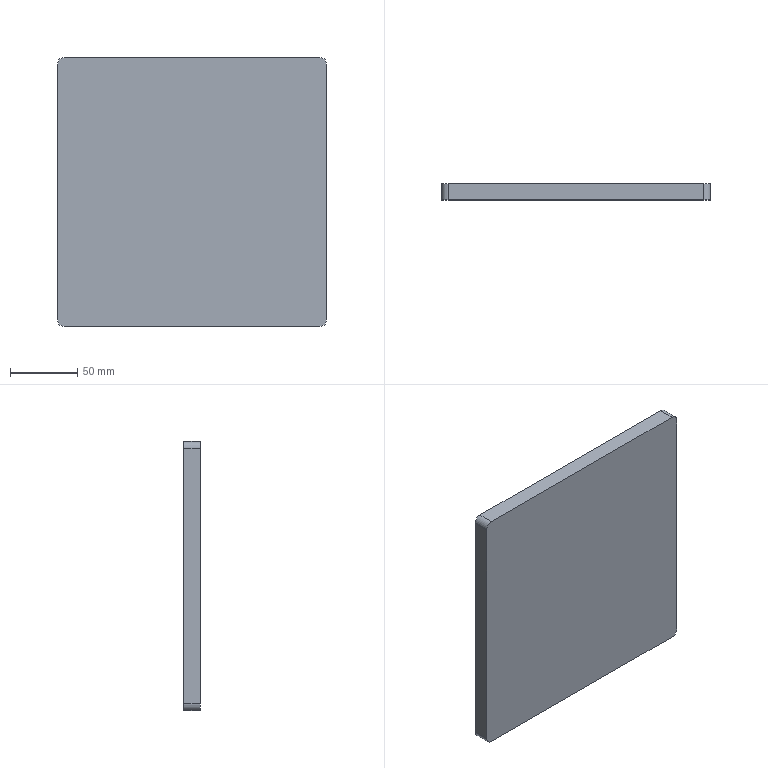Part | SolidWorks | features Cut 1, Extrusion 1, Fillet 1 | 1 solid | 30 faces | box 200 x 12 x 200 mm | volume 468015 mm3 | plane 18 | cylinder 12 | commonest cylinder face diameters 6.5 x8 10 x4
STEP:
#1=CARTESIAN_POINT('',(100.,12.,95.));
#2=VERTEX_POINT('',#1);
#3=CARTESIAN_POINT('',(100.,12.,-95.));
#4=VERTEX_POINT('',#3);
#5=CARTESIAN_POINT('',(100.,12.,-100.));
#6=DIRECTION('',(0.,0.,-1.));
#7=VECTOR('',#6,1000.);
#8=LINE('',#5,#7);
#9=EDGE_CURVE('',#2,#4,#8,.T.);
#10=ORIENTED_EDGE('',*,*,#9,.F.);
#11=CARTESIAN_POINT('',(100.,0.,95.));
#12=VERTEX_POINT('',#11);
#13=CARTESIAN_POINT('',(100.,12.,95.));
#14=DIRECTION('',(0.,-1.,0.));
#15=VECTOR('',#14,1000.);
#16=LINE('',#13,#15);
#17=EDGE_CURVE('',#2,#12,#16,.T.);
#18=ORIENTED_EDGE('',*,*,#17,.T.);
#19=CARTESIAN_POINT('',(100.,0.,-95.));
#20=VERTEX_POINT('',#19);
#21=CARTESIAN_POINT('',(100.,0.,-100.));
#22=DIRECTION('',(0.,0.,-1.));
#23=VECTOR('',#22,1000.);
#24=LINE('',#21,#23);
#25=EDGE_CURVE('',#12,#20,#24,.T.);
#26=ORIENTED_EDGE('',*,*,#25,.T.);
#27=CARTESIAN_POINT('',(100.,12.,-95.));
#28=DIRECTION('',(0.,1.,0.));
#29=VECTOR('',#28,1000.);
#30=LINE('',#27,#29);
#31=EDGE_CURVE('',#20,#4,#30,.T.);
#32=ORIENTED_EDGE('',*,*,#31,.T.);
#33=EDGE_LOOP('',(#10,#18,#26,#32));
#34=FACE_OUTER_BOUND('',#33,.T.);
#35=CARTESIAN_POINT('',(100.,12.,-100.));
#36=DIRECTION('',(-1.,0.,0.));
#37=DIRECTION('',(0.,0.,1.));
#38=AXIS2_PLACEMENT_3D('',#35,#36,#37);
#39=PLANE('',#38);
#40=ADVANCED_FACE('',(#34),#39,.F.);
#41=CARTESIAN_POINT('',(95.,12.,-100.));
#42=VERTEX_POINT('',#41);
#43=CARTESIAN_POINT('',(-95.,12.,-100.));
#44=VERTEX_POINT('',#43);
#45=CARTESIAN_POINT('',(-100.,12.,-100.));
#46=DIRECTION('',(-1.,0.,0.));
#47=VECTOR('',#46,1000.);
#48=LINE('',#45,#47);
#49=EDGE_CURVE('',#42,#44,#48,.T.);
#50=ORIENTED_EDGE('',*,*,#49,.F.);
#51=CARTESIAN_POINT('',(95.,0.,-100.));
#52=VERTEX_POINT('',#51);
#53=CARTESIAN_POINT('',(95.,12.,-100.));
#54=DIRECTION('',(0.,-1.,0.));
#55=VECTOR('',#54,1000.);
#56=LINE('',#53,#55);
#57=EDGE_CURVE('',#42,#52,#56,.T.);
#58=ORIENTED_EDGE('',*,*,#57,.T.);
#59=CARTESIAN_POINT('',(-95.,0.,-100.));
#60=VERTEX_POINT('',#59);
#61=CARTESIAN_POINT('',(-100.,0.,-100.));
#62=DIRECTION('',(-1.,0.,0.));
#63=VECTOR('',#62,1000.);
#64=LINE('',#61,#63);
#65=EDGE_CURVE('',#52,#60,#64,.T.);
#66=ORIENTED_EDGE('',*,*,#65,.T.);
#67=CARTESIAN_POINT('',(-95.,12.,-100.));
#68=DIRECTION('',(0.,1.,0.));
#69=VECTOR('',#68,1000.);
#70=LINE('',#67,#69);
#71=EDGE_CURVE('',#60,#44,#70,.T.);
#72=ORIENTED_EDGE('',*,*,#71,.T.);
#73=EDGE_LOOP('',(#50,#58,#66,#72));
#74=FACE_OUTER_BOUND('',#73,.T.);
#75=CARTESIAN_POINT('',(-100.,12.,-100.));
#76=DIRECTION('',(0.,0.,1.));
#77=DIRECTION('',(1.,0.,0.));
#78=AXIS2_PLACEMENT_3D('',#75,#76,#77);
#79=PLANE('',#78);
#80=ADVANCED_FACE('',(#74),#79,.F.);
#81=CARTESIAN_POINT('',(-100.,0.,-95.));
#82=VERTEX_POINT('',#81);
#83=CARTESIAN_POINT('',(-100.,0.,95.));
#84=VERTEX_POINT('',#83);
#85=CARTESIAN_POINT('',(-100.,0.,-100.));
#86=DIRECTION('',(0.,0.,1.));
#87=VECTOR('',#86,1000.);
#88=LINE('',#85,#87);
#89=EDGE_CURVE('',#82,#84,#88,.T.);
#90=ORIENTED_EDGE('',*,*,#89,.T.);
#91=CARTESIAN_POINT('',(-100.,12.,95.));
#92=VERTEX_POINT('',#91);
#93=CARTESIAN_POINT('',(-100.,12.,95.));
#94=DIRECTION('',(0.,1.,0.));
#95=VECTOR('',#94,1000.);
#96=LINE('',#93,#95);
#97=EDGE_CURVE('',#84,#92,#96,.T.);
#98=ORIENTED_EDGE('',*,*,#97,.T.);
#99=CARTESIAN_POINT('',(-100.,12.,-95.));
#100=VERTEX_POINT('',#99);
#101=CARTESIAN_POINT('',(-100.,12.,-100.));
#102=DIRECTION('',(0.,0.,1.));
#103=VECTOR('',#102,1000.);
#104=LINE('',#101,#103);
#105=EDGE_CURVE('',#100,#92,#104,.T.);
#106=ORIENTED_EDGE('',*,*,#105,.F.);
#107=CARTESIAN_POINT('',(-100.,12.,-95.));
#108=DIRECTION('',(0.,-1.,0.));
#109=VECTOR('',#108,1000.);
#110=LINE('',#107,#109);
#111=EDGE_CURVE('',#100,#82,#110,.T.);
#112=ORIENTED_EDGE('',*,*,#111,.T.);
#113=EDGE_LOOP('',(#90,#98,#106,#112));
#114=FACE_OUTER_BOUND('',#113,.T.);
#115=CARTESIAN_POINT('',(-100.,12.,-100.));
#116=DIRECTION('',(1.,0.,0.));
#117=DIRECTION('',(0.,0.,-1.));
#118=AXIS2_PLACEMENT_3D('',#115,#116,#117);
#119=PLANE('',#118);
#120=ADVANCED_FACE('',(#114),#119,.F.);
#121=CARTESIAN_POINT('',(-95.,12.,100.));
#122=VERTEX_POINT('',#121);
#123=CARTESIAN_POINT('',(95.,12.,100.));
#124=VERTEX_POINT('',#123);
#125=CARTESIAN_POINT('',(-100.,12.,100.));
#126=DIRECTION('',(1.,0.,0.));
#127=VECTOR('',#126,1000.);
#128=LINE('',#125,#127);
#129=EDGE_CURVE('',#122,#124,#128,.T.);
#130=ORIENTED_EDGE('',*,*,#129,.F.);
#131=CARTESIAN_POINT('',(-95.,0.,100.));
#132=VERTEX_POINT('',#131);
#133=CARTESIAN_POINT('',(-95.,12.,100.));
#134=DIRECTION('',(0.,-1.,0.));
#135=VECTOR('',#134,1000.);
#136=LINE('',#133,#135);
#137=EDGE_CURVE('',#122,#132,#136,.T.);
#138=ORIENTED_EDGE('',*,*,#137,.T.);
#139=CARTESIAN_POINT('',(95.,0.,100.));
#140=VERTEX_POINT('',#139);
#141=CARTESIAN_POINT('',(-100.,0.,100.));
#142=DIRECTION('',(1.,0.,0.));
#143=VECTOR('',#142,1000.);
#144=LINE('',#141,#143);
#145=EDGE_CURVE('',#132,#140,#144,.T.);
#146=ORIENTED_EDGE('',*,*,#145,.T.);
#147=CARTESIAN_POINT('',(95.,12.,100.));
#148=DIRECTION('',(0.,1.,0.));
#149=VECTOR('',#148,1000.);
#150=LINE('',#147,#149);
#151=EDGE_CURVE('',#140,#124,#150,.T.);
#152=ORIENTED_EDGE('',*,*,#151,.T.);
#153=EDGE_LOOP('',(#130,#138,#146,#152));
#154=FACE_OUTER_BOUND('',#153,.T.);
#155=CARTESIAN_POINT('',(-100.,12.,100.));
#156=DIRECTION('',(0.,0.,-1.));
#157=DIRECTION('',(-1.,0.,0.));
#158=AXIS2_PLACEMENT_3D('',#155,#156,#157);
#159=PLANE('',#158);
#160=ADVANCED_FACE('',(#154),#159,.F.);
#161=CARTESIAN_POINT('',(-90.,12.,80.125));
#162=VERTEX_POINT('',#161);
#163=CARTESIAN_POINT('',(-90.,12.,86.625));
#164=VERTEX_POINT('',#163);
#165=CARTESIAN_POINT('',(-90.,12.,83.375));
#166=DIRECTION('',(0.,1.,0.));
#167=DIRECTION('',(0.,0.,-1.));
#168=AXIS2_PLACEMENT_3D('',#165,#166,#167);
#169=CIRCLE('',#168,3.25);
#170=EDGE_CURVE('',#162,#164,#169,.T.);
#171=ORIENTED_EDGE('',*,*,#170,.F.);
#172=CARTESIAN_POINT('',(-70.,12.,80.125));
#173=VERTEX_POINT('',#172);
#174=CARTESIAN_POINT('',(-90.,12.,80.125));
#175=DIRECTION('',(-1.,0.,0.));
#176=VECTOR('',#175,1000.);
#177=LINE('',#174,#176);
#178=EDGE_CURVE('',#173,#162,#177,.T.);
#179=ORIENTED_EDGE('',*,*,#178,.F.);
#180=CARTESIAN_POINT('',(-70.,12.,86.625));
#181=VERTEX_POINT('',#180);
#182=CARTESIAN_POINT('',(-70.,12.,83.375));
#183=DIRECTION('',(0.,1.,0.));
#184=DIRECTION('',(0.,0.,-1.));
#185=AXIS2_PLACEMENT_3D('',#182,#183,#184);
#186=CIRCLE('',#185,3.25);
#187=EDGE_CURVE('',#181,#173,#186,.T.);
#188=ORIENTED_EDGE('',*,*,#187,.F.);
#189=CARTESIAN_POINT('',(-90.,12.,86.625));
#190=DIRECTION('',(1.,0.,0.));
#191=VECTOR('',#190,1000.);
#192=LINE('',#189,#191);
#193=EDGE_CURVE('',#164,#181,#192,.T.);
#194=ORIENTED_EDGE('',*,*,#193,.F.);
#195=EDGE_LOOP('',(#171,#179,#188,#194));
#196=FACE_BOUND('',#195,.T.);
#197=CARTESIAN_POINT('',(30.,12.,-88.25));
#198=VERTEX_POINT('',#197);
#199=CARTESIAN_POINT('',(30.,12.,-81.75));
#200=VERTEX_POINT('',#199);
#201=CARTESIAN_POINT('',(30.,12.,-85.));
#202=DIRECTION('',(0.,1.,0.));
#203=DIRECTION('',(0.,0.,1.));
#204=AXIS2_PLACEMENT_3D('',#201,#202,#203);
#205=CIRCLE('',#204,3.25);
#206=EDGE_CURVE('',#198,#200,#205,.T.);
#207=ORIENTED_EDGE('',*,*,#206,.F.);
#208=CARTESIAN_POINT('',(90.,12.,-88.25));
#209=VERTEX_POINT('',#208);
#210=CARTESIAN_POINT('',(30.,12.,-88.25));
#211=DIRECTION('',(-1.,0.,0.));
#212=VECTOR('',#211,1000.);
#213=LINE('',#210,#212);
#214=EDGE_CURVE('',#209,#198,#213,.T.);
#215=ORIENTED_EDGE('',*,*,#214,.F.);
#216=CARTESIAN_POINT('',(90.,12.,-81.75));
#217=VERTEX_POINT('',#216);
#218=CARTESIAN_POINT('',(90.,12.,-85.));
#219=DIRECTION('',(0.,1.,0.));
#220=DIRECTION('',(0.,0.,1.));
#221=AXIS2_PLACEMENT_3D('',#218,#219,#220);
#222=CIRCLE('',#221,3.25);
#223=EDGE_CURVE('',#217,#209,#222,.T.);
#224=ORIENTED_EDGE('',*,*,#223,.F.);
#225=CARTESIAN_POINT('',(30.,12.,-81.75));
#226=DIRECTION('',(1.,0.,0.));
#227=VECTOR('',#226,1000.);
#228=LINE('',#225,#227);
#229=EDGE_CURVE('',#200,#217,#228,.T.);
#230=ORIENTED_EDGE('',*,*,#229,.F.);
#231=EDGE_LOOP('',(#207,#215,#224,#230));
#232=FACE_BOUND('',#231,.T.);
#233=CARTESIAN_POINT('',(30.,12.,81.75));
#234=VERTEX_POINT('',#233);
#235=CARTESIAN_POINT('',(30.,12.,88.25));
#236=VERTEX_POINT('',#235);
#237=CARTESIAN_POINT('',(30.,12.,85.));
#238=DIRECTION('',(0.,1.,0.));
#239=DIRECTION('',(0.,0.,-1.));
#240=AXIS2_PLACEMENT_3D('',#237,#238,#239);
#241=CIRCLE('',#240,3.25);
#242=EDGE_CURVE('',#234,#236,#241,.T.);
#243=ORIENTED_EDGE('',*,*,#242,.F.);
#244=CARTESIAN_POINT('',(90.,12.,81.75));
#245=VERTEX_POINT('',#244);
#246=CARTESIAN_POINT('',(30.,12.,81.75));
#247=DIRECTION('',(-1.,0.,0.));
#248=VECTOR('',#247,1000.);
#249=LINE('',#246,#248);
#250=EDGE_CURVE('',#245,#234,#249,.T.);
#251=ORIENTED_EDGE('',*,*,#250,.F.);
#252=CARTESIAN_POINT('',(90.,12.,88.25));
#253=VERTEX_POINT('',#252);
#254=CARTESIAN_POINT('',(90.,12.,85.));
#255=DIRECTION('',(0.,1.,0.));
#256=DIRECTION('',(0.,0.,-1.));
#257=AXIS2_PLACEMENT_3D('',#254,#255,#256);
#258=CIRCLE('',#257,3.25);
#259=EDGE_CURVE('',#253,#245,#258,.T.);
#260=ORIENTED_EDGE('',*,*,#259,.F.);
#261=CARTESIAN_POINT('',(30.,12.,88.25));
#262=DIRECTION('',(1.,0.,0.));
#263=VECTOR('',#262,1000.);
#264=LINE('',#261,#263);
#265=EDGE_CURVE('',#236,#253,#264,.T.);
#266=ORIENTED_EDGE('',*,*,#265,.F.);
#267=EDGE_LOOP('',(#243,#251,#260,#266));
#268=FACE_BOUND('',#267,.T.);
#269=CARTESIAN_POINT('',(-90.,12.,-86.625));
#270=VERTEX_POINT('',#269);
#271=CARTESIAN_POINT('',(-90.,12.,-80.125));
#272=VERTEX_POINT('',#271);
#273=CARTESIAN_POINT('',(-90.,12.,-83.375));
#274=DIRECTION('',(0.,1.,0.));
#275=DIRECTION('',(0.,0.,1.));
#276=AXIS2_PLACEMENT_3D('',#273,#274,#275);
#277=CIRCLE('',#276,3.25);
#278=EDGE_CURVE('',#270,#272,#277,.T.);
#279=ORIENTED_EDGE('',*,*,#278,.F.);
#280=CARTESIAN_POINT('',(-70.,12.,-86.625));
#281=VERTEX_POINT('',#280);
#282=CARTESIAN_POINT('',(-90.,12.,-86.625));
#283=DIRECTION('',(-1.,0.,0.));
#284=VECTOR('',#283,1000.);
#285=LINE('',#282,#284);
#286=EDGE_CURVE('',#281,#270,#285,.T.);
#287=ORIENTED_EDGE('',*,*,#286,.F.);
#288=CARTESIAN_POINT('',(-70.,12.,-80.125));
#289=VERTEX_POINT('',#288);
#290=CARTESIAN_POINT('',(-70.,12.,-83.375));
#291=DIRECTION('',(0.,1.,0.));
#292=DIRECTION('',(0.,0.,1.));
#293=AXIS2_PLACEMENT_3D('',#290,#291,#292);
#294=CIRCLE('',#293,3.25);
#295=EDGE_CURVE('',#289,#281,#294,.T.);
#296=ORIENTED_EDGE('',*,*,#295,.F.);
#297=CARTESIAN_POINT('',(-90.,12.,-80.125));
#298=DIRECTION('',(1.,0.,0.));
#299=VECTOR('',#298,1000.);
#300=LINE('',#297,#299);
#301=EDGE_CURVE('',#272,#289,#300,.T.);
#302=ORIENTED_EDGE('',*,*,#301,.F.);
#303=EDGE_LOOP('',(#279,#287,#296,#302));
#304=FACE_BOUND('',#303,.T.);
#305=ORIENTED_EDGE('',*,*,#105,.T.);
#306=CARTESIAN_POINT('',(-95.,12.,95.));
#307=DIRECTION('',(0.,1.,0.));
#308=DIRECTION('',(0.,0.,1.));
#309=AXIS2_PLACEMENT_3D('',#306,#307,#308);
#310=CIRCLE('',#309,5.);
#311=EDGE_CURVE('',#92,#122,#310,.T.);
#312=ORIENTED_EDGE('',*,*,#311,.T.);
#313=ORIENTED_EDGE('',*,*,#129,.T.);
#314=CARTESIAN_POINT('',(95.,12.,95.));
#315=DIRECTION('',(0.,1.,0.));
#316=DIRECTION('',(0.,0.,1.));
#317=AXIS2_PLACEMENT_3D('',#314,#315,#316);
#318=CIRCLE('',#317,5.);
#319=EDGE_CURVE('',#124,#2,#318,.T.);
#320=ORIENTED_EDGE('',*,*,#319,.T.);
#321=ORIENTED_EDGE('',*,*,#9,.T.);
#322=CARTESIAN_POINT('',(95.,12.,-95.));
#323=DIRECTION('',(0.,1.,0.));
#324=DIRECTION('',(0.,0.,1.));
#325=AXIS2_PLACEMENT_3D('',#322,#323,#324);
#326=CIRCLE('',#325,5.);
#327=EDGE_CURVE('',#4,#42,#326,.T.);
#328=ORIENTED_EDGE('',*,*,#327,.T.);
#329=ORIENTED_EDGE('',*,*,#49,.T.);
#330=CARTESIAN_POINT('',(-95.,12.,-95.));
#331=DIRECTION('',(0.,1.,0.));
#332=DIRECTION('',(0.,0.,1.));
#333=AXIS2_PLACEMENT_3D('',#330,#331,#332);
#334=CIRCLE('',#333,5.);
#335=EDGE_CURVE('',#44,#100,#334,.T.);
#336=ORIENTED_EDGE('',*,*,#335,.T.);
#337=EDGE_LOOP('',(#305,#312,#313,#320,#321,#328,#329,#336));
#338=FACE_OUTER_BOUND('',#337,.T.);
#339=CARTESIAN_POINT('',(0.,12.,0.));
#340=DIRECTION('',(0.,1.,0.));
#341=DIRECTION('',(0.,0.,1.));
#342=AXIS2_PLACEMENT_3D('',#339,#340,#341);
#343=PLANE('',#342);
#344=ADVANCED_FACE('',(#196,#232,#268,#304,#338),#343,.T.);
#345=ORIENTED_EDGE('',*,*,#145,.F.);
#346=CARTESIAN_POINT('',(-95.,0.,95.));
#347=DIRECTION('',(0.,-1.,0.));
#348=DIRECTION('',(0.,0.,1.));
#349=AXIS2_PLACEMENT_3D('',#346,#347,#348);
#350=CIRCLE('',#349,5.);
#351=EDGE_CURVE('',#132,#84,#350,.T.);
#352=ORIENTED_EDGE('',*,*,#351,.T.);
#353=ORIENTED_EDGE('',*,*,#89,.F.);
#354=CARTESIAN_POINT('',(-95.,0.,-95.));
#355=DIRECTION('',(0.,-1.,0.));
#356=DIRECTION('',(0.,0.,1.));
#357=AXIS2_PLACEMENT_3D('',#354,#355,#356);
#358=CIRCLE('',#357,5.);
#359=EDGE_CURVE('',#82,#60,#358,.T.);
#360=ORIENTED_EDGE('',*,*,#359,.T.);
#361=ORIENTED_EDGE('',*,*,#65,.F.);
#362=CARTESIAN_POINT('',(95.,0.,-95.));
#363=DIRECTION('',(0.,-1.,0.));
#364=DIRECTION('',(0.,0.,1.));
#365=AXIS2_PLACEMENT_3D('',#362,#363,#364);
#366=CIRCLE('',#365,5.);
#367=EDGE_CURVE('',#52,#20,#366,.T.);
#368=ORIENTED_EDGE('',*,*,#367,.T.);
#369=ORIENTED_EDGE('',*,*,#25,.F.);
#370=CARTESIAN_POINT('',(95.,0.,95.));
#371=DIRECTION('',(0.,-1.,0.));
#372=DIRECTION('',(0.,0.,1.));
#373=AXIS2_PLACEMENT_3D('',#370,#371,#372);
#374=CIRCLE('',#373,5.);
#375=EDGE_CURVE('',#12,#140,#374,.T.);
#376=ORIENTED_EDGE('',*,*,#375,.T.);
#377=EDGE_LOOP('',(#345,#352,#353,#360,#361,#368,#369,#376));
#378=FACE_OUTER_BOUND('',#377,.T.);
#379=CARTESIAN_POINT('',(0.,0.,0.));
#380=DIRECTION('',(0.,1.,0.));
#381=DIRECTION('',(0.,0.,1.));
#382=AXIS2_PLACEMENT_3D('',#379,#380,#381);
#383=PLANE('',#382);
#384=ADVANCED_FACE('',(#378),#383,.F.);
#385=ORIENTED_EDGE('',*,*,#311,.F.);
#386=ORIENTED_EDGE('',*,*,#97,.F.);
#387=ORIENTED_EDGE('',*,*,#351,.F.);
#388=ORIENTED_EDGE('',*,*,#137,.F.);
#389=EDGE_LOOP('',(#385,#386,#387,#388));
#390=FACE_OUTER_BOUND('',#389,.T.);
#391=CARTESIAN_POINT('',(-95.,12.,95.));
#392=DIRECTION('',(0.,-1.,0.));
#393=DIRECTION('',(0.,0.,-1.));
#394=AXIS2_PLACEMENT_3D('',#391,#392,#393);
#395=CYLINDRICAL_SURFACE('',#394,5.);
#396=ADVANCED_FACE('',(#390),#395,.T.);
#397=ORIENTED_EDGE('',*,*,#319,.F.);
#398=ORIENTED_EDGE('',*,*,#151,.F.);
#399=ORIENTED_EDGE('',*,*,#375,.F.);
#400=ORIENTED_EDGE('',*,*,#17,.F.);
#401=EDGE_LOOP('',(#397,#398,#399,#400));
#402=FACE_OUTER_BOUND('',#401,.T.);
#403=CARTESIAN_POINT('',(95.,12.,95.));
#404=DIRECTION('',(0.,-1.,0.));
#405=DIRECTION('',(0.,0.,-1.));
#406=AXIS2_PLACEMENT_3D('',#403,#404,#405);
#407=CYLINDRICAL_SURFACE('',#406,5.);
#408=ADVANCED_FACE('',(#402),#407,.T.);
#409=ORIENTED_EDGE('',*,*,#327,.F.);
#410=ORIENTED_EDGE('',*,*,#31,.F.);
#411=ORIENTED_EDGE('',*,*,#367,.F.);
#412=ORIENTED_EDGE('',*,*,#57,.F.);
#413=EDGE_LOOP('',(#409,#410,#411,#412));
#414=FACE_OUTER_BOUND('',#413,.T.);
#415=CARTESIAN_POINT('',(95.,12.,-95.));
#416=DIRECTION('',(0.,-1.,0.));
#417=DIRECTION('',(0.,0.,-1.));
#418=AXIS2_PLACEMENT_3D('',#415,#416,#417);
#419=CYLINDRICAL_SURFACE('',#418,5.);
#420=ADVANCED_FACE('',(#414),#419,.T.);
#421=ORIENTED_EDGE('',*,*,#335,.F.);
#422=ORIENTED_EDGE('',*,*,#71,.F.);
#423=ORIENTED_EDGE('',*,*,#359,.F.);
#424=ORIENTED_EDGE('',*,*,#111,.F.);
#425=EDGE_LOOP('',(#421,#422,#423,#424));
#426=FACE_OUTER_BOUND('',#425,.T.);
#427=CARTESIAN_POINT('',(-95.,12.,-95.));
#428=DIRECTION('',(0.,-1.,0.));
#429=DIRECTION('',(0.,0.,-1.));
#430=AXIS2_PLACEMENT_3D('',#427,#428,#429);
#431=CYLINDRICAL_SURFACE('',#430,5.);
#432=ADVANCED_FACE('',(#426),#431,.T.);
#433=ORIENTED_EDGE('',*,*,#278,.T.);
#434=CARTESIAN_POINT('',(-90.,2.,-80.125));
#435=VERTEX_POINT('',#434);
#436=CARTESIAN_POINT('',(-90.,2.,-80.125));
#437=DIRECTION('',(0.,1.,0.));
#438=VECTOR('',#437,1000.);
#439=LINE('',#436,#438);
#440=EDGE_CURVE('',#435,#272,#439,.T.);
#441=ORIENTED_EDGE('',*,*,#440,.F.);
#442=CARTESIAN_POINT('',(-90.,2.,-86.625));
#443=VERTEX_POINT('',#442);
#444=CARTESIAN_POINT('',(-90.,2.,-83.375));
#445=DIRECTION('',(0.,1.,0.));
#446=DIRECTION('',(0.,0.,1.));
#447=AXIS2_PLACEMENT_3D('',#444,#445,#446);
#448=CIRCLE('',#447,3.25);
#449=EDGE_CURVE('',#443,#435,#448,.T.);
#450=ORIENTED_EDGE('',*,*,#449,.F.);
#451=CARTESIAN_POINT('',(-90.,2.,-86.625));
#452=DIRECTION('',(0.,1.,0.));
#453=VECTOR('',#452,1000.);
#454=LINE('',#451,#453);
#455=EDGE_CURVE('',#443,#270,#454,.T.);
#456=ORIENTED_EDGE('',*,*,#455,.T.);
#457=EDGE_LOOP('',(#433,#441,#450,#456));
#458=FACE_OUTER_BOUND('',#457,.T.);
#459=CARTESIAN_POINT('',(-90.,2.,-83.375));
#460=DIRECTION('',(0.,1.,0.));
#461=DIRECTION('',(0.,0.,1.));
#462=AXIS2_PLACEMENT_3D('',#459,#460,#461);
#463=CYLINDRICAL_SURFACE('',#462,3.25);
#464=ADVANCED_FACE('',(#458),#463,.F.);
#465=ORIENTED_EDGE('',*,*,#286,.T.);
#466=ORIENTED_EDGE('',*,*,#455,.F.);
#467=CARTESIAN_POINT('',(-70.,2.,-86.625));
#468=VERTEX_POINT('',#467);
#469=CARTESIAN_POINT('',(-90.,2.,-86.625));
#470=DIRECTION('',(-1.,0.,0.));
#471=VECTOR('',#470,1000.);
#472=LINE('',#469,#471);
#473=EDGE_CURVE('',#468,#443,#472,.T.);
#474=ORIENTED_EDGE('',*,*,#473,.F.);
#475=CARTESIAN_POINT('',(-70.,2.,-86.625));
#476=DIRECTION('',(0.,1.,0.));
#477=VECTOR('',#476,1000.);
#478=LINE('',#475,#477);
#479=EDGE_CURVE('',#468,#281,#478,.T.);
#480=ORIENTED_EDGE('',*,*,#479,.T.);
#481=EDGE_LOOP('',(#465,#466,#474,#480));
#482=FACE_OUTER_BOUND('',#481,.T.);
#483=CARTESIAN_POINT('',(-90.,2.,-86.625));
#484=DIRECTION('',(0.,0.,-1.));
#485=DIRECTION('',(-1.,0.,0.));
#486=AXIS2_PLACEMENT_3D('',#483,#484,#485);
#487=PLANE('',#486);
#488=ADVANCED_FACE('',(#482),#487,.F.);
#489=ORIENTED_EDGE('',*,*,#295,.T.);
#490=ORIENTED_EDGE('',*,*,#479,.F.);
#491=CARTESIAN_POINT('',(-70.,2.,-80.125));
#492=VERTEX_POINT('',#491);
#493=CARTESIAN_POINT('',(-70.,2.,-83.375));
#494=DIRECTION('',(0.,1.,0.));
#495=DIRECTION('',(0.,0.,1.));
#496=AXIS2_PLACEMENT_3D('',#493,#494,#495);
#497=CIRCLE('',#496,3.25);
#498=EDGE_CURVE('',#492,#468,#497,.T.);
#499=ORIENTED_EDGE('',*,*,#498,.F.);
#500=CARTESIAN_POINT('',(-70.,2.,-80.125));
#501=DIRECTION('',(0.,1.,0.));
#502=VECTOR('',#501,1000.);
#503=LINE('',#500,#502);
#504=EDGE_CURVE('',#492,#289,#503,.T.);
#505=ORIENTED_EDGE('',*,*,#504,.T.);
#506=EDGE_LOOP('',(#489,#490,#499,#505));
#507=FACE_OUTER_BOUND('',#506,.T.);
#508=CARTESIAN_POINT('',(-70.,2.,-83.375));
#509=DIRECTION('',(0.,1.,0.));
#510=DIRECTION('',(0.,0.,1.));
#511=AXIS2_PLACEMENT_3D('',#508,#509,#510);
#512=CYLINDRICAL_SURFACE('',#511,3.25);
#513=ADVANCED_FACE('',(#507),#512,.F.);
#514=ORIENTED_EDGE('',*,*,#301,.T.);
#515=ORIENTED_EDGE('',*,*,#504,.F.);
#516=CARTESIAN_POINT('',(-90.,2.,-80.125));
#517=DIRECTION('',(1.,0.,0.));
#518=VECTOR('',#517,1000.);
#519=LINE('',#516,#518);
#520=EDGE_CURVE('',#435,#492,#519,.T.);
#521=ORIENTED_EDGE('',*,*,#520,.F.);
#522=ORIENTED_EDGE('',*,*,#440,.T.);
#523=EDGE_LOOP('',(#514,#515,#521,#522));
#524=FACE_OUTER_BOUND('',#523,.T.);
#525=CARTESIAN_POINT('',(-90.,2.,-80.125));
#526=DIRECTION('',(0.,0.,1.));
#527=DIRECTION('',(1.,0.,0.));
#528=AXIS2_PLACEMENT_3D('',#525,#526,#527);
#529=PLANE('',#528);
#530=ADVANCED_FACE('',(#524),#529,.F.);
#531=ORIENTED_EDGE('',*,*,#449,.T.);
#532=ORIENTED_EDGE('',*,*,#520,.T.);
#533=ORIENTED_EDGE('',*,*,#498,.T.);
#534=ORIENTED_EDGE('',*,*,#473,.T.);
#535=EDGE_LOOP('',(#531,#532,#533,#534));
#536=FACE_OUTER_BOUND('',#535,.T.);
#537=CARTESIAN_POINT('',(-90.,2.,-83.375));
#538=DIRECTION('',(0.,1.,0.));
#539=DIRECTION('',(0.,0.,1.));
#540=AXIS2_PLACEMENT_3D('',#537,#538,#539);
#541=PLANE('',#540);
#542=ADVANCED_FACE('',(#536),#541,.T.);
#543=ORIENTED_EDGE('',*,*,#242,.T.);
#544=CARTESIAN_POINT('',(30.,2.,88.25));
#545=VERTEX_POINT('',#544);
#546=CARTESIAN_POINT('',(30.,2.,88.25));
#547=DIRECTION('',(0.,1.,0.));
#548=VECTOR('',#547,1000.);
#549=LINE('',#546,#548);
#550=EDGE_CURVE('',#545,#236,#549,.T.);
#551=ORIENTED_EDGE('',*,*,#550,.F.);
#552=CARTESIAN_POINT('',(30.,2.,81.75));
#553=VERTEX_POINT('',#552);
#554=CARTESIAN_POINT('',(30.,2.,85.));
#555=DIRECTION('',(0.,1.,0.));
#556=DIRECTION('',(0.,0.,-1.));
#557=AXIS2_PLACEMENT_3D('',#554,#555,#556);
#558=CIRCLE('',#557,3.25);
#559=EDGE_CURVE('',#553,#545,#558,.T.);
#560=ORIENTED_EDGE('',*,*,#559,.F.);
#561=CARTESIAN_POINT('',(30.,2.,81.75));
#562=DIRECTION('',(0.,1.,0.));
#563=VECTOR('',#562,1000.);
#564=LINE('',#561,#563);
#565=EDGE_CURVE('',#553,#234,#564,.T.);
#566=ORIENTED_EDGE('',*,*,#565,.T.);
#567=EDGE_LOOP('',(#543,#551,#560,#566));
#568=FACE_OUTER_BOUND('',#567,.T.);
#569=CARTESIAN_POINT('',(30.,2.,85.));
#570=DIRECTION('',(0.,1.,0.));
#571=DIRECTION('',(0.,0.,1.));
#572=AXIS2_PLACEMENT_3D('',#569,#570,#571);
#573=CYLINDRICAL_SURFACE('',#572,3.25);
#574=ADVANCED_FACE('',(#568),#573,.F.);
#575=ORIENTED_EDGE('',*,*,#250,.T.);
#576=ORIENTED_EDGE('',*,*,#565,.F.);
#577=CARTESIAN_POINT('',(90.,2.,81.75));
#578=VERTEX_POINT('',#577);
#579=CARTESIAN_POINT('',(30.,2.,81.75));
#580=DIRECTION('',(-1.,0.,0.));
#581=VECTOR('',#580,1000.);
#582=LINE('',#579,#581);
#583=EDGE_CURVE('',#578,#553,#582,.T.);
#584=ORIENTED_EDGE('',*,*,#583,.F.);
#585=CARTESIAN_POINT('',(90.,2.,81.75));
#586=DIRECTION('',(0.,1.,0.));
#587=VECTOR('',#586,1000.);
#588=LINE('',#585,#587);
#589=EDGE_CURVE('',#578,#245,#588,.T.);
#590=ORIENTED_EDGE('',*,*,#589,.T.);
#591=EDGE_LOOP('',(#575,#576,#584,#590));
#592=FACE_OUTER_BOUND('',#591,.T.);
#593=CARTESIAN_POINT('',(30.,2.,81.75));
#594=DIRECTION('',(0.,0.,-1.));
#595=DIRECTION('',(-1.,0.,0.));
#596=AXIS2_PLACEMENT_3D('',#593,#594,#595);
#597=PLANE('',#596);
#598=ADVANCED_FACE('',(#592),#597,.F.);
#599=ORIENTED_EDGE('',*,*,#259,.T.);
#600=ORIENTED_EDGE('',*,*,#589,.F.);
#601=CARTESIAN_POINT('',(90.,2.,88.25));
#602=VERTEX_POINT('',#601);
#603=CARTESIAN_POINT('',(90.,2.,85.));
#604=DIRECTION('',(0.,1.,0.));
#605=DIRECTION('',(0.,0.,-1.));
#606=AXIS2_PLACEMENT_3D('',#603,#604,#605);
#607=CIRCLE('',#606,3.25);
#608=EDGE_CURVE('',#602,#578,#607,.T.);
#609=ORIENTED_EDGE('',*,*,#608,.F.);
#610=CARTESIAN_POINT('',(90.,2.,88.25));
#611=DIRECTION('',(0.,1.,0.));
#612=VECTOR('',#611,1000.);
#613=LINE('',#610,#612);
#614=EDGE_CURVE('',#602,#253,#613,.T.);
#615=ORIENTED_EDGE('',*,*,#614,.T.);
#616=EDGE_LOOP('',(#599,#600,#609,#615));
#617=FACE_OUTER_BOUND('',#616,.T.);
#618=CARTESIAN_POINT('',(90.,2.,85.));
#619=DIRECTION('',(0.,1.,0.));
#620=DIRECTION('',(0.,0.,1.));
#621=AXIS2_PLACEMENT_3D('',#618,#619,#620);
#622=CYLINDRICAL_SURFACE('',#621,3.25);
#623=ADVANCED_FACE('',(#617),#622,.F.);
#624=ORIENTED_EDGE('',*,*,#265,.T.);
#625=ORIENTED_EDGE('',*,*,#614,.F.);
#626=CARTESIAN_POINT('',(30.,2.,88.25));
#627=DIRECTION('',(1.,0.,0.));
#628=VECTOR('',#627,1000.);
#629=LINE('',#626,#628);
#630=EDGE_CURVE('',#545,#602,#629,.T.);
#631=ORIENTED_EDGE('',*,*,#630,.F.);
#632=ORIENTED_EDGE('',*,*,#550,.T.);
#633=EDGE_LOOP('',(#624,#625,#631,#632));
#634=FACE_OUTER_BOUND('',#633,.T.);
#635=CARTESIAN_POINT('',(30.,2.,88.25));
#636=DIRECTION('',(0.,0.,1.));
#637=DIRECTION('',(1.,0.,0.));
#638=AXIS2_PLACEMENT_3D('',#635,#636,#637);
#639=PLANE('',#638);
#640=ADVANCED_FACE('',(#634),#639,.F.);
#641=ORIENTED_EDGE('',*,*,#559,.T.);
#642=ORIENTED_EDGE('',*,*,#630,.T.);
#643=ORIENTED_EDGE('',*,*,#608,.T.);
#644=ORIENTED_EDGE('',*,*,#583,.T.);
#645=EDGE_LOOP('',(#641,#642,#643,#644));
#646=FACE_OUTER_BOUND('',#645,.T.);
#647=CARTESIAN_POINT('',(30.,2.,85.));
#648=DIRECTION('',(0.,-1.,0.));
#649=DIRECTION('',(0.,0.,-1.));
#650=AXIS2_PLACEMENT_3D('',#647,#648,#649);
#651=PLANE('',#650);
#652=ADVANCED_FACE('',(#646),#651,.F.);
#653=ORIENTED_EDGE('',*,*,#206,.T.);
#654=CARTESIAN_POINT('',(30.,2.,-81.75));
#655=VERTEX_POINT('',#654);
#656=CARTESIAN_POINT('',(30.,2.,-81.75));
#657=DIRECTION('',(0.,1.,0.));
#658=VECTOR('',#657,1000.);
#659=LINE('',#656,#658);
#660=EDGE_CURVE('',#655,#200,#659,.T.);
#661=ORIENTED_EDGE('',*,*,#660,.F.);
#662=CARTESIAN_POINT('',(30.,2.,-88.25));
#663=VERTEX_POINT('',#662);
#664=CARTESIAN_POINT('',(30.,2.,-85.));
#665=DIRECTION('',(0.,1.,0.));
#666=DIRECTION('',(0.,0.,1.));
#667=AXIS2_PLACEMENT_3D('',#664,#665,#666);
#668=CIRCLE('',#667,3.25);
#669=EDGE_CURVE('',#663,#655,#668,.T.);
#670=ORIENTED_EDGE('',*,*,#669,.F.);
#671=CARTESIAN_POINT('',(30.,2.,-88.25));
#672=DIRECTION('',(0.,1.,0.));
#673=VECTOR('',#672,1000.);
#674=LINE('',#671,#673);
#675=EDGE_CURVE('',#663,#198,#674,.T.);
#676=ORIENTED_EDGE('',*,*,#675,.T.);
#677=EDGE_LOOP('',(#653,#661,#670,#676));
#678=FACE_OUTER_BOUND('',#677,.T.);
#679=CARTESIAN_POINT('',(30.,2.,-85.));
#680=DIRECTION('',(0.,1.,0.));
#681=DIRECTION('',(0.,0.,1.));
#682=AXIS2_PLACEMENT_3D('',#679,#680,#681);
#683=CYLINDRICAL_SURFACE('',#682,3.25);
#684=ADVANCED_FACE('',(#678),#683,.F.);
#685=ORIENTED_EDGE('',*,*,#214,.T.);
#686=ORIENTED_EDGE('',*,*,#675,.F.);
#687=CARTESIAN_POINT('',(90.,2.,-88.25));
#688=VERTEX_POINT('',#687);
#689=CARTESIAN_POINT('',(30.,2.,-88.25));
#690=DIRECTION('',(-1.,0.,0.));
#691=VECTOR('',#690,1000.);
#692=LINE('',#689,#691);
#693=EDGE_CURVE('',#688,#663,#692,.T.);
#694=ORIENTED_EDGE('',*,*,#693,.F.);
#695=CARTESIAN_POINT('',(90.,2.,-88.25));
#696=DIRECTION('',(0.,1.,0.));
#697=VECTOR('',#696,1000.);
#698=LINE('',#695,#697);
#699=EDGE_CURVE('',#688,#209,#698,.T.);
#700=ORIENTED_EDGE('',*,*,#699,.T.);
#701=EDGE_LOOP('',(#685,#686,#694,#700));
#702=FACE_OUTER_BOUND('',#701,.T.);
#703=CARTESIAN_POINT('',(30.,2.,-88.25));
#704=DIRECTION('',(0.,0.,-1.));
#705=DIRECTION('',(-1.,0.,0.));
#706=AXIS2_PLACEMENT_3D('',#703,#704,#705);
#707=PLANE('',#706);
#708=ADVANCED_FACE('',(#702),#707,.F.);
#709=ORIENTED_EDGE('',*,*,#223,.T.);
#710=ORIENTED_EDGE('',*,*,#699,.F.);
#711=CARTESIAN_POINT('',(90.,2.,-81.75));
#712=VERTEX_POINT('',#711);
#713=CARTESIAN_POINT('',(90.,2.,-85.));
#714=DIRECTION('',(0.,1.,0.));
#715=DIRECTION('',(0.,0.,1.));
#716=AXIS2_PLACEMENT_3D('',#713,#714,#715);
#717=CIRCLE('',#716,3.25);
#718=EDGE_CURVE('',#712,#688,#717,.T.);
#719=ORIENTED_EDGE('',*,*,#718,.F.);
#720=CARTESIAN_POINT('',(90.,2.,-81.75));
#721=DIRECTION('',(0.,1.,0.));
#722=VECTOR('',#721,1000.);
#723=LINE('',#720,#722);
#724=EDGE_CURVE('',#712,#217,#723,.T.);
#725=ORIENTED_EDGE('',*,*,#724,.T.);
#726=EDGE_LOOP('',(#709,#710,#719,#725));
#727=FACE_OUTER_BOUND('',#726,.T.);
#728=CARTESIAN_POINT('',(90.,2.,-85.));
#729=DIRECTION('',(0.,1.,0.));
#730=DIRECTION('',(0.,0.,1.));
#731=AXIS2_PLACEMENT_3D('',#728,#729,#730);
#732=CYLINDRICAL_SURFACE('',#731,3.25);
#733=ADVANCED_FACE('',(#727),#732,.F.);
#734=ORIENTED_EDGE('',*,*,#229,.T.);
#735=ORIENTED_EDGE('',*,*,#724,.F.);
#736=CARTESIAN_POINT('',(30.,2.,-81.75));
#737=DIRECTION('',(1.,0.,0.));
#738=VECTOR('',#737,1000.);
#739=LINE('',#736,#738);
#740=EDGE_CURVE('',#655,#712,#739,.T.);
#741=ORIENTED_EDGE('',*,*,#740,.F.);
#742=ORIENTED_EDGE('',*,*,#660,.T.);
#743=EDGE_LOOP('',(#734,#735,#741,#742));
#744=FACE_OUTER_BOUND('',#743,.T.);
#745=CARTESIAN_POINT('',(30.,2.,-81.75));
#746=DIRECTION('',(0.,0.,1.));
#747=DIRECTION('',(1.,0.,0.));
#748=AXIS2_PLACEMENT_3D('',#745,#746,#747);
#749=PLANE('',#748);
#750=ADVANCED_FACE('',(#744),#749,.F.);
#751=ORIENTED_EDGE('',*,*,#669,.T.);
#752=ORIENTED_EDGE('',*,*,#740,.T.);
#753=ORIENTED_EDGE('',*,*,#718,.T.);
#754=ORIENTED_EDGE('',*,*,#693,.T.);
#755=EDGE_LOOP('',(#751,#752,#753,#754));
#756=FACE_OUTER_BOUND('',#755,.T.);
#757=CARTESIAN_POINT('',(30.,2.,-85.));
#758=DIRECTION('',(0.,1.,0.));
#759=DIRECTION('',(0.,0.,1.));
#760=AXIS2_PLACEMENT_3D('',#757,#758,#759);
#761=PLANE('',#760);
#762=ADVANCED_FACE('',(#756),#761,.T.);
#763=ORIENTED_EDGE('',*,*,#170,.T.);
#764=CARTESIAN_POINT('',(-90.,2.,86.625));
#765=VERTEX_POINT('',#764);
#766=CARTESIAN_POINT('',(-90.,2.,86.625));
#767=DIRECTION('',(0.,1.,0.));
#768=VECTOR('',#767,1000.);
#769=LINE('',#766,#768);
#770=EDGE_CURVE('',#765,#164,#769,.T.);
#771=ORIENTED_EDGE('',*,*,#770,.F.);
#772=CARTESIAN_POINT('',(-90.,2.,80.125));
#773=VERTEX_POINT('',#772);
#774=CARTESIAN_POINT('',(-90.,2.,83.375));
#775=DIRECTION('',(0.,1.,0.));
#776=DIRECTION('',(0.,0.,-1.));
#777=AXIS2_PLACEMENT_3D('',#774,#775,#776);
#778=CIRCLE('',#777,3.25);
#779=EDGE_CURVE('',#773,#765,#778,.T.);
#780=ORIENTED_EDGE('',*,*,#779,.F.);
#781=CARTESIAN_POINT('',(-90.,2.,80.125));
#782=DIRECTION('',(0.,1.,0.));
#783=VECTOR('',#782,1000.);
#784=LINE('',#781,#783);
#785=EDGE_CURVE('',#773,#162,#784,.T.);
#786=ORIENTED_EDGE('',*,*,#785,.T.);
#787=EDGE_LOOP('',(#763,#771,#780,#786));
#788=FACE_OUTER_BOUND('',#787,.T.);
#789=CARTESIAN_POINT('',(-90.,2.,83.375));
#790=DIRECTION('',(0.,1.,0.));
#791=DIRECTION('',(0.,0.,1.));
#792=AXIS2_PLACEMENT_3D('',#789,#790,#791);
#793=CYLINDRICAL_SURFACE('',#792,3.25);
#794=ADVANCED_FACE('',(#788),#793,.F.);
#795=ORIENTED_EDGE('',*,*,#178,.T.);
#796=ORIENTED_EDGE('',*,*,#785,.F.);
#797=CARTESIAN_POINT('',(-70.,2.,80.125));
#798=VERTEX_POINT('',#797);
#799=CARTESIAN_POINT('',(-90.,2.,80.125));
#800=DIRECTION('',(-1.,0.,0.));
#801=VECTOR('',#800,1000.);
#802=LINE('',#799,#801);
#803=EDGE_CURVE('',#798,#773,#802,.T.);
#804=ORIENTED_EDGE('',*,*,#803,.F.);
#805=CARTESIAN_POINT('',(-70.,2.,80.125));
#806=DIRECTION('',(0.,1.,0.));
#807=VECTOR('',#806,1000.);
#808=LINE('',#805,#807);
#809=EDGE_CURVE('',#798,#173,#808,.T.);
#810=ORIENTED_EDGE('',*,*,#809,.T.);
#811=EDGE_LOOP('',(#795,#796,#804,#810));
#812=FACE_OUTER_BOUND('',#811,.T.);
#813=CARTESIAN_POINT('',(-90.,2.,80.125));
#814=DIRECTION('',(0.,0.,-1.));
#815=DIRECTION('',(-1.,0.,0.));
#816=AXIS2_PLACEMENT_3D('',#813,#814,#815);
#817=PLANE('',#816);
#818=ADVANCED_FACE('',(#812),#817,.F.);
#819=ORIENTED_EDGE('',*,*,#187,.T.);
#820=ORIENTED_EDGE('',*,*,#809,.F.);
#821=CARTESIAN_POINT('',(-70.,2.,86.625));
#822=VERTEX_POINT('',#821);
#823=CARTESIAN_POINT('',(-70.,2.,83.375));
#824=DIRECTION('',(0.,1.,0.));
#825=DIRECTION('',(0.,0.,-1.));
#826=AXIS2_PLACEMENT_3D('',#823,#824,#825);
#827=CIRCLE('',#826,3.25);
#828=EDGE_CURVE('',#822,#798,#827,.T.);
#829=ORIENTED_EDGE('',*,*,#828,.F.);
#830=CARTESIAN_POINT('',(-70.,2.,86.625));
#831=DIRECTION('',(0.,1.,0.));
#832=VECTOR('',#831,1000.);
#833=LINE('',#830,#832);
#834=EDGE_CURVE('',#822,#181,#833,.T.);
#835=ORIENTED_EDGE('',*,*,#834,.T.);
#836=EDGE_LOOP('',(#819,#820,#829,#835));
#837=FACE_OUTER_BOUND('',#836,.T.);
#838=CARTESIAN_POINT('',(-70.,2.,83.375));
#839=DIRECTION('',(0.,1.,0.));
#840=DIRECTION('',(0.,0.,1.));
#841=AXIS2_PLACEMENT_3D('',#838,#839,#840);
#842=CYLINDRICAL_SURFACE('',#841,3.25);
#843=ADVANCED_FACE('',(#837),#842,.F.);
#844=ORIENTED_EDGE('',*,*,#193,.T.);
#845=ORIENTED_EDGE('',*,*,#834,.F.);
#846=CARTESIAN_POINT('',(-90.,2.,86.625));
#847=DIRECTION('',(1.,0.,0.));
#848=VECTOR('',#847,1000.);
#849=LINE('',#846,#848);
#850=EDGE_CURVE('',#765,#822,#849,.T.);
#851=ORIENTED_EDGE('',*,*,#850,.F.);
#852=ORIENTED_EDGE('',*,*,#770,.T.);
#853=EDGE_LOOP('',(#844,#845,#851,#852));
#854=FACE_OUTER_BOUND('',#853,.T.);
#855=CARTESIAN_POINT('',(-90.,2.,86.625));
#856=DIRECTION('',(0.,0.,1.));
#857=DIRECTION('',(1.,0.,0.));
#858=AXIS2_PLACEMENT_3D('',#855,#856,#857);
#859=PLANE('',#858);
#860=ADVANCED_FACE('',(#854),#859,.F.);
#861=ORIENTED_EDGE('',*,*,#779,.T.);
#862=ORIENTED_EDGE('',*,*,#850,.T.);
#863=ORIENTED_EDGE('',*,*,#828,.T.);
#864=ORIENTED_EDGE('',*,*,#803,.T.);
#865=EDGE_LOOP('',(#861,#862,#863,#864));
#866=FACE_OUTER_BOUND('',#865,.T.);
#867=CARTESIAN_POINT('',(-90.,2.,83.375));
#868=DIRECTION('',(0.,-1.,0.));
#869=DIRECTION('',(0.,0.,-1.));
#870=AXIS2_PLACEMENT_3D('',#867,#868,#869);
#871=PLANE('',#870);
#872=ADVANCED_FACE('',(#866),#871,.F.);
#873=CLOSED_SHELL('',(#40,#80,#120,#160,#344,#384,#396,#408,#420,#432,#464,#488,#513,#530,#542,#574,#598,#623,#640,#652,#684,#708,#733,#750,#762,#794,#818,#843,#860,#872));
#874=MANIFOLD_SOLID_BREP('',#873);
#875=CARTESIAN_POINT('',(0.,0.,0.));
#876=DIRECTION('',(0.,0.,1.));
#877=DIRECTION('',(1.,0.,0.));
#878=AXIS2_PLACEMENT_3D('',#875,#876,#877);
#879=(LENGTH_UNIT()NAMED_UNIT(*)SI_UNIT(.MILLI.,.METRE.));
#880=UNCERTAINTY_MEASURE_WITH_UNIT(LENGTH_MEASURE(0.00001),#879,'','');
#881=(NAMED_UNIT(*)PLANE_ANGLE_UNIT()SI_UNIT($,.RADIAN.));
#882=(NAMED_UNIT(*)SI_UNIT($,.STERADIAN.)SOLID_ANGLE_UNIT());
#883=(GEOMETRIC_REPRESENTATION_CONTEXT(3)GLOBAL_UNCERTAINTY_ASSIGNED_CONTEXT((#880))GLOBAL_UNIT_ASSIGNED_CONTEXT((#879,#881,#882))REPRESENTATION_CONTEXT('',''));
#884=ADVANCED_BREP_SHAPE_REPRESENTATION('',(#874,#878),#883);